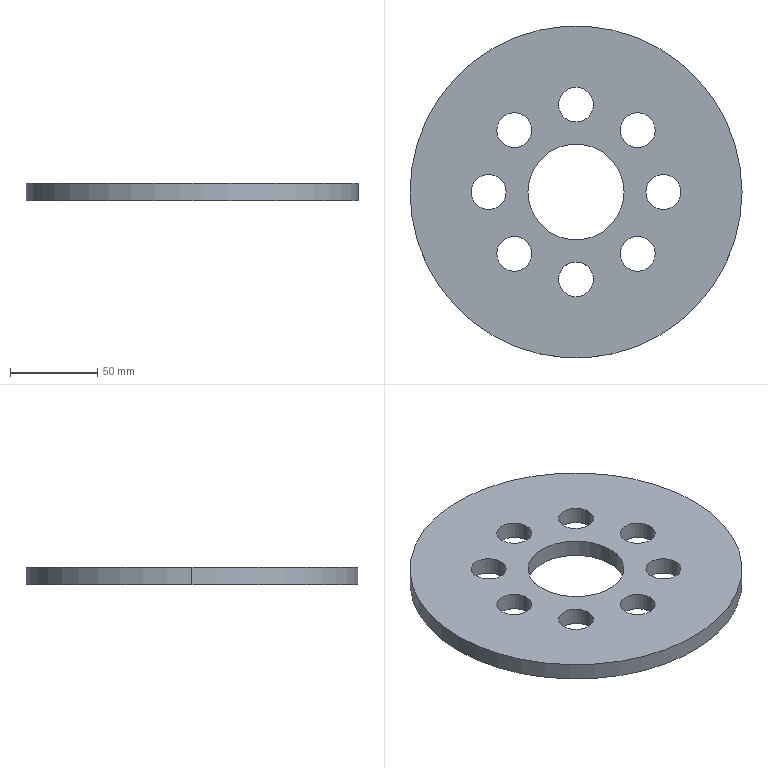Part | SolidWorks | features CirPattern 1, Cut 1, Extrusion 1 | 1 solid | 22 faces | box 190 x 190 x 10 mm | volume 234638 mm3 | cylinder 20 | plane 2 | commonest cylinder face diameters 20 x16 55 x2 190 x2
STEP:
#1=CARTESIAN_POINT('',(-10.,50.,0.));
#2=VERTEX_POINT('',#1);
#3=CARTESIAN_POINT('',(10.,50.,0.));
#4=VERTEX_POINT('',#3);
#5=CARTESIAN_POINT('',(0.,50.,0.));
#6=DIRECTION('',(0.,0.,1.));
#7=DIRECTION('',(0.,1.,0.));
#8=AXIS2_PLACEMENT_3D('',#5,#6,#7);
#9=CIRCLE('',#8,10.);
#10=EDGE_CURVE('',#2,#4,#9,.T.);
#11=ORIENTED_EDGE('',*,*,#10,.F.);
#12=CARTESIAN_POINT('',(-10.,50.,10.));
#13=VERTEX_POINT('',#12);
#14=CARTESIAN_POINT('',(-10.,50.,0.));
#15=DIRECTION('',(0.,0.,1.));
#16=VECTOR('',#15,1000.);
#17=LINE('',#14,#16);
#18=EDGE_CURVE('',#2,#13,#17,.T.);
#19=ORIENTED_EDGE('',*,*,#18,.T.);
#20=CARTESIAN_POINT('',(10.,50.,10.));
#21=VERTEX_POINT('',#20);
#22=CARTESIAN_POINT('',(0.,50.,10.));
#23=DIRECTION('',(0.,0.,1.));
#24=DIRECTION('',(1.,0.,0.));
#25=AXIS2_PLACEMENT_3D('',#22,#23,#24);
#26=CIRCLE('',#25,10.);
#27=EDGE_CURVE('',#13,#21,#26,.T.);
#28=ORIENTED_EDGE('',*,*,#27,.T.);
#29=CARTESIAN_POINT('',(10.,50.,0.));
#30=DIRECTION('',(0.,0.,1.));
#31=VECTOR('',#30,1000.);
#32=LINE('',#29,#31);
#33=EDGE_CURVE('',#4,#21,#32,.T.);
#34=ORIENTED_EDGE('',*,*,#33,.F.);
#35=EDGE_LOOP('',(#11,#19,#28,#34));
#36=FACE_OUTER_BOUND('',#35,.T.);
#37=CARTESIAN_POINT('',(0.,50.,0.));
#38=DIRECTION('',(0.,0.,1.));
#39=DIRECTION('',(1.,0.,0.));
#40=AXIS2_PLACEMENT_3D('',#37,#38,#39);
#41=CYLINDRICAL_SURFACE('',#40,10.);
#42=ADVANCED_FACE('',(#36),#41,.F.);
#43=CARTESIAN_POINT('',(-45.355,35.355,0.));
#44=VERTEX_POINT('',#43);
#45=CARTESIAN_POINT('',(-25.355,35.355,0.));
#46=VERTEX_POINT('',#45);
#47=CARTESIAN_POINT('',(-35.355,35.355,0.));
#48=DIRECTION('',(0.,0.,1.));
#49=DIRECTION('',(-0.7071,0.7071,0.));
#50=AXIS2_PLACEMENT_3D('',#47,#48,#49);
#51=CIRCLE('',#50,10.);
#52=EDGE_CURVE('',#44,#46,#51,.T.);
#53=ORIENTED_EDGE('',*,*,#52,.F.);
#54=CARTESIAN_POINT('',(-45.355,35.355,10.));
#55=VERTEX_POINT('',#54);
#56=CARTESIAN_POINT('',(-45.355,35.355,0.));
#57=DIRECTION('',(0.,0.,1.));
#58=VECTOR('',#57,1000.);
#59=LINE('',#56,#58);
#60=EDGE_CURVE('',#44,#55,#59,.T.);
#61=ORIENTED_EDGE('',*,*,#60,.T.);
#62=CARTESIAN_POINT('',(-25.355,35.355,10.));
#63=VERTEX_POINT('',#62);
#64=CARTESIAN_POINT('',(-35.355,35.355,10.));
#65=DIRECTION('',(0.,0.,1.));
#66=DIRECTION('',(1.,0.,0.));
#67=AXIS2_PLACEMENT_3D('',#64,#65,#66);
#68=CIRCLE('',#67,10.);
#69=EDGE_CURVE('',#55,#63,#68,.T.);
#70=ORIENTED_EDGE('',*,*,#69,.T.);
#71=CARTESIAN_POINT('',(-25.355,35.355,0.));
#72=DIRECTION('',(0.,0.,1.));
#73=VECTOR('',#72,1000.);
#74=LINE('',#71,#73);
#75=EDGE_CURVE('',#46,#63,#74,.T.);
#76=ORIENTED_EDGE('',*,*,#75,.F.);
#77=EDGE_LOOP('',(#53,#61,#70,#76));
#78=FACE_OUTER_BOUND('',#77,.T.);
#79=CARTESIAN_POINT('',(-35.355,35.355,0.));
#80=DIRECTION('',(0.,0.,1.));
#81=DIRECTION('',(1.,0.,0.));
#82=AXIS2_PLACEMENT_3D('',#79,#80,#81);
#83=CYLINDRICAL_SURFACE('',#82,10.);
#84=ADVANCED_FACE('',(#78),#83,.F.);
#85=CARTESIAN_POINT('',(-60.,0.,0.));
#86=VERTEX_POINT('',#85);
#87=CARTESIAN_POINT('',(-40.,0.,0.));
#88=VERTEX_POINT('',#87);
#89=CARTESIAN_POINT('',(-50.,0.,0.));
#90=DIRECTION('',(0.,0.,1.));
#91=DIRECTION('',(-1.,0.,0.));
#92=AXIS2_PLACEMENT_3D('',#89,#90,#91);
#93=CIRCLE('',#92,10.);
#94=EDGE_CURVE('',#86,#88,#93,.T.);
#95=ORIENTED_EDGE('',*,*,#94,.F.);
#96=CARTESIAN_POINT('',(-60.,0.,10.));
#97=VERTEX_POINT('',#96);
#98=CARTESIAN_POINT('',(-60.,0.,0.));
#99=DIRECTION('',(0.,0.,1.));
#100=VECTOR('',#99,1000.);
#101=LINE('',#98,#100);
#102=EDGE_CURVE('',#86,#97,#101,.T.);
#103=ORIENTED_EDGE('',*,*,#102,.T.);
#104=CARTESIAN_POINT('',(-40.,0.,10.));
#105=VERTEX_POINT('',#104);
#106=CARTESIAN_POINT('',(-50.,0.,10.));
#107=DIRECTION('',(0.,0.,1.));
#108=DIRECTION('',(1.,0.,0.));
#109=AXIS2_PLACEMENT_3D('',#106,#107,#108);
#110=CIRCLE('',#109,10.);
#111=EDGE_CURVE('',#97,#105,#110,.T.);
#112=ORIENTED_EDGE('',*,*,#111,.T.);
#113=CARTESIAN_POINT('',(-40.,0.,0.));
#114=DIRECTION('',(0.,0.,1.));
#115=VECTOR('',#114,1000.);
#116=LINE('',#113,#115);
#117=EDGE_CURVE('',#88,#105,#116,.T.);
#118=ORIENTED_EDGE('',*,*,#117,.F.);
#119=EDGE_LOOP('',(#95,#103,#112,#118));
#120=FACE_OUTER_BOUND('',#119,.T.);
#121=CARTESIAN_POINT('',(-50.,0.,0.));
#122=DIRECTION('',(0.,0.,1.));
#123=DIRECTION('',(1.,0.,0.));
#124=AXIS2_PLACEMENT_3D('',#121,#122,#123);
#125=CYLINDRICAL_SURFACE('',#124,10.);
#126=ADVANCED_FACE('',(#120),#125,.F.);
#127=CARTESIAN_POINT('',(-45.355,-35.355,0.));
#128=VERTEX_POINT('',#127);
#129=CARTESIAN_POINT('',(-25.355,-35.355,0.));
#130=VERTEX_POINT('',#129);
#131=CARTESIAN_POINT('',(-35.355,-35.355,0.));
#132=DIRECTION('',(0.,0.,1.));
#133=DIRECTION('',(-0.7071,-0.7071,0.));
#134=AXIS2_PLACEMENT_3D('',#131,#132,#133);
#135=CIRCLE('',#134,10.);
#136=EDGE_CURVE('',#128,#130,#135,.T.);
#137=ORIENTED_EDGE('',*,*,#136,.F.);
#138=CARTESIAN_POINT('',(-45.355,-35.355,10.));
#139=VERTEX_POINT('',#138);
#140=CARTESIAN_POINT('',(-45.355,-35.355,0.));
#141=DIRECTION('',(0.,0.,1.));
#142=VECTOR('',#141,1000.);
#143=LINE('',#140,#142);
#144=EDGE_CURVE('',#128,#139,#143,.T.);
#145=ORIENTED_EDGE('',*,*,#144,.T.);
#146=CARTESIAN_POINT('',(-25.355,-35.355,10.));
#147=VERTEX_POINT('',#146);
#148=CARTESIAN_POINT('',(-35.355,-35.355,10.));
#149=DIRECTION('',(0.,0.,1.));
#150=DIRECTION('',(1.,0.,0.));
#151=AXIS2_PLACEMENT_3D('',#148,#149,#150);
#152=CIRCLE('',#151,10.);
#153=EDGE_CURVE('',#139,#147,#152,.T.);
#154=ORIENTED_EDGE('',*,*,#153,.T.);
#155=CARTESIAN_POINT('',(-25.355,-35.355,0.));
#156=DIRECTION('',(0.,0.,1.));
#157=VECTOR('',#156,1000.);
#158=LINE('',#155,#157);
#159=EDGE_CURVE('',#130,#147,#158,.T.);
#160=ORIENTED_EDGE('',*,*,#159,.F.);
#161=EDGE_LOOP('',(#137,#145,#154,#160));
#162=FACE_OUTER_BOUND('',#161,.T.);
#163=CARTESIAN_POINT('',(-35.355,-35.355,0.));
#164=DIRECTION('',(0.,0.,1.));
#165=DIRECTION('',(1.,0.,0.));
#166=AXIS2_PLACEMENT_3D('',#163,#164,#165);
#167=CYLINDRICAL_SURFACE('',#166,10.);
#168=ADVANCED_FACE('',(#162),#167,.F.);
#169=CARTESIAN_POINT('',(-10.,-50.,0.));
#170=VERTEX_POINT('',#169);
#171=CARTESIAN_POINT('',(10.,-50.,0.));
#172=VERTEX_POINT('',#171);
#173=CARTESIAN_POINT('',(0.,-50.,0.));
#174=DIRECTION('',(0.,0.,1.));
#175=DIRECTION('',(0.,-1.,0.));
#176=AXIS2_PLACEMENT_3D('',#173,#174,#175);
#177=CIRCLE('',#176,10.);
#178=EDGE_CURVE('',#170,#172,#177,.T.);
#179=ORIENTED_EDGE('',*,*,#178,.F.);
#180=CARTESIAN_POINT('',(-10.,-50.,10.));
#181=VERTEX_POINT('',#180);
#182=CARTESIAN_POINT('',(-10.,-50.,0.));
#183=DIRECTION('',(0.,0.,1.));
#184=VECTOR('',#183,1000.);
#185=LINE('',#182,#184);
#186=EDGE_CURVE('',#170,#181,#185,.T.);
#187=ORIENTED_EDGE('',*,*,#186,.T.);
#188=CARTESIAN_POINT('',(10.,-50.,10.));
#189=VERTEX_POINT('',#188);
#190=CARTESIAN_POINT('',(0.,-50.,10.));
#191=DIRECTION('',(0.,0.,1.));
#192=DIRECTION('',(1.,0.,0.));
#193=AXIS2_PLACEMENT_3D('',#190,#191,#192);
#194=CIRCLE('',#193,10.);
#195=EDGE_CURVE('',#181,#189,#194,.T.);
#196=ORIENTED_EDGE('',*,*,#195,.T.);
#197=CARTESIAN_POINT('',(10.,-50.,0.));
#198=DIRECTION('',(0.,0.,1.));
#199=VECTOR('',#198,1000.);
#200=LINE('',#197,#199);
#201=EDGE_CURVE('',#172,#189,#200,.T.);
#202=ORIENTED_EDGE('',*,*,#201,.F.);
#203=EDGE_LOOP('',(#179,#187,#196,#202));
#204=FACE_OUTER_BOUND('',#203,.T.);
#205=CARTESIAN_POINT('',(0.,-50.,0.));
#206=DIRECTION('',(0.,0.,1.));
#207=DIRECTION('',(1.,0.,0.));
#208=AXIS2_PLACEMENT_3D('',#205,#206,#207);
#209=CYLINDRICAL_SURFACE('',#208,10.);
#210=ADVANCED_FACE('',(#204),#209,.F.);
#211=CARTESIAN_POINT('',(25.355,-35.355,0.));
#212=VERTEX_POINT('',#211);
#213=CARTESIAN_POINT('',(45.355,-35.355,0.));
#214=VERTEX_POINT('',#213);
#215=CARTESIAN_POINT('',(35.355,-35.355,0.));
#216=DIRECTION('',(0.,0.,1.));
#217=DIRECTION('',(0.7071,-0.7071,0.));
#218=AXIS2_PLACEMENT_3D('',#215,#216,#217);
#219=CIRCLE('',#218,10.);
#220=EDGE_CURVE('',#212,#214,#219,.T.);
#221=ORIENTED_EDGE('',*,*,#220,.F.);
#222=CARTESIAN_POINT('',(25.355,-35.355,10.));
#223=VERTEX_POINT('',#222);
#224=CARTESIAN_POINT('',(25.355,-35.355,0.));
#225=DIRECTION('',(0.,0.,1.));
#226=VECTOR('',#225,1000.);
#227=LINE('',#224,#226);
#228=EDGE_CURVE('',#212,#223,#227,.T.);
#229=ORIENTED_EDGE('',*,*,#228,.T.);
#230=CARTESIAN_POINT('',(45.355,-35.355,10.));
#231=VERTEX_POINT('',#230);
#232=CARTESIAN_POINT('',(35.355,-35.355,10.));
#233=DIRECTION('',(0.,0.,1.));
#234=DIRECTION('',(1.,0.,0.));
#235=AXIS2_PLACEMENT_3D('',#232,#233,#234);
#236=CIRCLE('',#235,10.);
#237=EDGE_CURVE('',#223,#231,#236,.T.);
#238=ORIENTED_EDGE('',*,*,#237,.T.);
#239=CARTESIAN_POINT('',(45.355,-35.355,0.));
#240=DIRECTION('',(0.,0.,1.));
#241=VECTOR('',#240,1000.);
#242=LINE('',#239,#241);
#243=EDGE_CURVE('',#214,#231,#242,.T.);
#244=ORIENTED_EDGE('',*,*,#243,.F.);
#245=EDGE_LOOP('',(#221,#229,#238,#244));
#246=FACE_OUTER_BOUND('',#245,.T.);
#247=CARTESIAN_POINT('',(35.355,-35.355,0.));
#248=DIRECTION('',(0.,0.,1.));
#249=DIRECTION('',(1.,0.,0.));
#250=AXIS2_PLACEMENT_3D('',#247,#248,#249);
#251=CYLINDRICAL_SURFACE('',#250,10.);
#252=ADVANCED_FACE('',(#246),#251,.F.);
#253=CARTESIAN_POINT('',(25.355,35.355,0.));
#254=VERTEX_POINT('',#253);
#255=CARTESIAN_POINT('',(45.355,35.355,0.));
#256=VERTEX_POINT('',#255);
#257=CARTESIAN_POINT('',(35.355,35.355,0.));
#258=DIRECTION('',(0.,0.,1.));
#259=DIRECTION('',(0.7071,0.7071,0.));
#260=AXIS2_PLACEMENT_3D('',#257,#258,#259);
#261=CIRCLE('',#260,10.);
#262=EDGE_CURVE('',#254,#256,#261,.T.);
#263=ORIENTED_EDGE('',*,*,#262,.F.);
#264=CARTESIAN_POINT('',(25.355,35.355,10.));
#265=VERTEX_POINT('',#264);
#266=CARTESIAN_POINT('',(25.355,35.355,0.));
#267=DIRECTION('',(0.,0.,1.));
#268=VECTOR('',#267,1000.);
#269=LINE('',#266,#268);
#270=EDGE_CURVE('',#254,#265,#269,.T.);
#271=ORIENTED_EDGE('',*,*,#270,.T.);
#272=CARTESIAN_POINT('',(45.355,35.355,10.));
#273=VERTEX_POINT('',#272);
#274=CARTESIAN_POINT('',(35.355,35.355,10.));
#275=DIRECTION('',(0.,0.,1.));
#276=DIRECTION('',(1.,0.,0.));
#277=AXIS2_PLACEMENT_3D('',#274,#275,#276);
#278=CIRCLE('',#277,10.);
#279=EDGE_CURVE('',#265,#273,#278,.T.);
#280=ORIENTED_EDGE('',*,*,#279,.T.);
#281=CARTESIAN_POINT('',(45.355,35.355,0.));
#282=DIRECTION('',(0.,0.,1.));
#283=VECTOR('',#282,1000.);
#284=LINE('',#281,#283);
#285=EDGE_CURVE('',#256,#273,#284,.T.);
#286=ORIENTED_EDGE('',*,*,#285,.F.);
#287=EDGE_LOOP('',(#263,#271,#280,#286));
#288=FACE_OUTER_BOUND('',#287,.T.);
#289=CARTESIAN_POINT('',(35.355,35.355,0.));
#290=DIRECTION('',(0.,0.,1.));
#291=DIRECTION('',(1.,0.,0.));
#292=AXIS2_PLACEMENT_3D('',#289,#290,#291);
#293=CYLINDRICAL_SURFACE('',#292,10.);
#294=ADVANCED_FACE('',(#288),#293,.F.);
#295=CARTESIAN_POINT('',(40.,0.,0.));
#296=VERTEX_POINT('',#295);
#297=CARTESIAN_POINT('',(60.,0.,0.));
#298=VERTEX_POINT('',#297);
#299=CARTESIAN_POINT('',(50.,0.,0.));
#300=DIRECTION('',(0.,0.,1.));
#301=DIRECTION('',(1.,0.,0.));
#302=AXIS2_PLACEMENT_3D('',#299,#300,#301);
#303=CIRCLE('',#302,10.);
#304=EDGE_CURVE('',#296,#298,#303,.T.);
#305=ORIENTED_EDGE('',*,*,#304,.F.);
#306=CARTESIAN_POINT('',(40.,0.,10.));
#307=VERTEX_POINT('',#306);
#308=CARTESIAN_POINT('',(40.,0.,0.));
#309=DIRECTION('',(0.,0.,1.));
#310=VECTOR('',#309,1000.);
#311=LINE('',#308,#310);
#312=EDGE_CURVE('',#296,#307,#311,.T.);
#313=ORIENTED_EDGE('',*,*,#312,.T.);
#314=CARTESIAN_POINT('',(60.,0.,10.));
#315=VERTEX_POINT('',#314);
#316=CARTESIAN_POINT('',(50.,0.,10.));
#317=DIRECTION('',(0.,0.,1.));
#318=DIRECTION('',(1.,0.,0.));
#319=AXIS2_PLACEMENT_3D('',#316,#317,#318);
#320=CIRCLE('',#319,10.);
#321=EDGE_CURVE('',#307,#315,#320,.T.);
#322=ORIENTED_EDGE('',*,*,#321,.T.);
#323=CARTESIAN_POINT('',(60.,0.,0.));
#324=DIRECTION('',(0.,0.,1.));
#325=VECTOR('',#324,1000.);
#326=LINE('',#323,#325);
#327=EDGE_CURVE('',#298,#315,#326,.T.);
#328=ORIENTED_EDGE('',*,*,#327,.F.);
#329=EDGE_LOOP('',(#305,#313,#322,#328));
#330=FACE_OUTER_BOUND('',#329,.T.);
#331=CARTESIAN_POINT('',(50.,0.,0.));
#332=DIRECTION('',(0.,0.,1.));
#333=DIRECTION('',(1.,0.,0.));
#334=AXIS2_PLACEMENT_3D('',#331,#332,#333);
#335=CYLINDRICAL_SURFACE('',#334,10.);
#336=ADVANCED_FACE('',(#330),#335,.F.);
#337=CARTESIAN_POINT('',(-27.5,0.,10.));
#338=VERTEX_POINT('',#337);
#339=CARTESIAN_POINT('',(27.5,0.,10.));
#340=VERTEX_POINT('',#339);
#341=CARTESIAN_POINT('',(0.,0.,10.));
#342=DIRECTION('',(0.,0.,1.));
#343=DIRECTION('',(1.,0.,0.));
#344=AXIS2_PLACEMENT_3D('',#341,#342,#343);
#345=CIRCLE('',#344,27.5);
#346=EDGE_CURVE('',#338,#340,#345,.T.);
#347=ORIENTED_EDGE('',*,*,#346,.T.);
#348=CARTESIAN_POINT('',(27.5,0.,0.));
#349=VERTEX_POINT('',#348);
#350=CARTESIAN_POINT('',(27.5,0.,10.));
#351=DIRECTION('',(0.,0.,-1.));
#352=VECTOR('',#351,1000.);
#353=LINE('',#350,#352);
#354=EDGE_CURVE('',#340,#349,#353,.T.);
#355=ORIENTED_EDGE('',*,*,#354,.T.);
#356=CARTESIAN_POINT('',(-27.5,0.,0.));
#357=VERTEX_POINT('',#356);
#358=CARTESIAN_POINT('',(0.,0.,0.));
#359=DIRECTION('',(0.,0.,1.));
#360=DIRECTION('',(1.,0.,0.));
#361=AXIS2_PLACEMENT_3D('',#358,#359,#360);
#362=CIRCLE('',#361,27.5);
#363=EDGE_CURVE('',#357,#349,#362,.T.);
#364=ORIENTED_EDGE('',*,*,#363,.F.);
#365=CARTESIAN_POINT('',(-27.5,0.,10.));
#366=DIRECTION('',(0.,0.,-1.));
#367=VECTOR('',#366,1000.);
#368=LINE('',#365,#367);
#369=EDGE_CURVE('',#338,#357,#368,.T.);
#370=ORIENTED_EDGE('',*,*,#369,.F.);
#371=EDGE_LOOP('',(#347,#355,#364,#370));
#372=FACE_OUTER_BOUND('',#371,.T.);
#373=CARTESIAN_POINT('',(0.,0.,10.));
#374=DIRECTION('',(0.,0.,-1.));
#375=DIRECTION('',(-1.,0.,0.));
#376=AXIS2_PLACEMENT_3D('',#373,#374,#375);
#377=CYLINDRICAL_SURFACE('',#376,27.5);
#378=ADVANCED_FACE('',(#372),#377,.F.);
#379=CARTESIAN_POINT('',(95.,0.,10.));
#380=VERTEX_POINT('',#379);
#381=CARTESIAN_POINT('',(-95.,0.,10.));
#382=VERTEX_POINT('',#381);
#383=CARTESIAN_POINT('',(0.,0.,10.));
#384=DIRECTION('',(0.,0.,1.));
#385=DIRECTION('',(1.,0.,0.));
#386=AXIS2_PLACEMENT_3D('',#383,#384,#385);
#387=CIRCLE('',#386,95.);
#388=EDGE_CURVE('',#380,#382,#387,.T.);
#389=ORIENTED_EDGE('',*,*,#388,.F.);
#390=CARTESIAN_POINT('',(95.,0.,0.));
#391=VERTEX_POINT('',#390);
#392=CARTESIAN_POINT('',(95.,0.,10.));
#393=DIRECTION('',(0.,0.,-1.));
#394=VECTOR('',#393,1000.);
#395=LINE('',#392,#394);
#396=EDGE_CURVE('',#380,#391,#395,.T.);
#397=ORIENTED_EDGE('',*,*,#396,.T.);
#398=CARTESIAN_POINT('',(-95.,0.,0.));
#399=VERTEX_POINT('',#398);
#400=CARTESIAN_POINT('',(0.,0.,0.));
#401=DIRECTION('',(0.,0.,1.));
#402=DIRECTION('',(1.,0.,0.));
#403=AXIS2_PLACEMENT_3D('',#400,#401,#402);
#404=CIRCLE('',#403,95.);
#405=EDGE_CURVE('',#391,#399,#404,.T.);
#406=ORIENTED_EDGE('',*,*,#405,.T.);
#407=CARTESIAN_POINT('',(-95.,0.,10.));
#408=DIRECTION('',(0.,0.,-1.));
#409=VECTOR('',#408,1000.);
#410=LINE('',#407,#409);
#411=EDGE_CURVE('',#382,#399,#410,.T.);
#412=ORIENTED_EDGE('',*,*,#411,.F.);
#413=EDGE_LOOP('',(#389,#397,#406,#412));
#414=FACE_OUTER_BOUND('',#413,.T.);
#415=CARTESIAN_POINT('',(0.,0.,10.));
#416=DIRECTION('',(0.,0.,-1.));
#417=DIRECTION('',(-1.,0.,0.));
#418=AXIS2_PLACEMENT_3D('',#415,#416,#417);
#419=CYLINDRICAL_SURFACE('',#418,95.);
#420=ADVANCED_FACE('',(#414),#419,.T.);
#421=CARTESIAN_POINT('',(0.,50.,10.));
#422=DIRECTION('',(0.,0.,1.));
#423=DIRECTION('',(1.,0.,0.));
#424=AXIS2_PLACEMENT_3D('',#421,#422,#423);
#425=CIRCLE('',#424,10.);
#426=EDGE_CURVE('',#21,#13,#425,.T.);
#427=ORIENTED_EDGE('',*,*,#426,.F.);
#428=ORIENTED_EDGE('',*,*,#27,.F.);
#429=EDGE_LOOP('',(#427,#428));
#430=FACE_BOUND('',#429,.T.);
#431=CARTESIAN_POINT('',(-35.355,35.355,10.));
#432=DIRECTION('',(0.,0.,1.));
#433=DIRECTION('',(1.,0.,0.));
#434=AXIS2_PLACEMENT_3D('',#431,#432,#433);
#435=CIRCLE('',#434,10.);
#436=EDGE_CURVE('',#63,#55,#435,.T.);
#437=ORIENTED_EDGE('',*,*,#436,.F.);
#438=ORIENTED_EDGE('',*,*,#69,.F.);
#439=EDGE_LOOP('',(#437,#438));
#440=FACE_BOUND('',#439,.T.);
#441=CARTESIAN_POINT('',(-50.,0.,10.));
#442=DIRECTION('',(0.,0.,1.));
#443=DIRECTION('',(1.,0.,0.));
#444=AXIS2_PLACEMENT_3D('',#441,#442,#443);
#445=CIRCLE('',#444,10.);
#446=EDGE_CURVE('',#105,#97,#445,.T.);
#447=ORIENTED_EDGE('',*,*,#446,.F.);
#448=ORIENTED_EDGE('',*,*,#111,.F.);
#449=EDGE_LOOP('',(#447,#448));
#450=FACE_BOUND('',#449,.T.);
#451=CARTESIAN_POINT('',(-35.355,-35.355,10.));
#452=DIRECTION('',(0.,0.,1.));
#453=DIRECTION('',(1.,0.,0.));
#454=AXIS2_PLACEMENT_3D('',#451,#452,#453);
#455=CIRCLE('',#454,10.);
#456=EDGE_CURVE('',#147,#139,#455,.T.);
#457=ORIENTED_EDGE('',*,*,#456,.F.);
#458=ORIENTED_EDGE('',*,*,#153,.F.);
#459=EDGE_LOOP('',(#457,#458));
#460=FACE_BOUND('',#459,.T.);
#461=CARTESIAN_POINT('',(0.,-50.,10.));
#462=DIRECTION('',(0.,0.,1.));
#463=DIRECTION('',(1.,0.,0.));
#464=AXIS2_PLACEMENT_3D('',#461,#462,#463);
#465=CIRCLE('',#464,10.);
#466=EDGE_CURVE('',#189,#181,#465,.T.);
#467=ORIENTED_EDGE('',*,*,#466,.F.);
#468=ORIENTED_EDGE('',*,*,#195,.F.);
#469=EDGE_LOOP('',(#467,#468));
#470=FACE_BOUND('',#469,.T.);
#471=CARTESIAN_POINT('',(35.355,-35.355,10.));
#472=DIRECTION('',(0.,0.,1.));
#473=DIRECTION('',(1.,0.,0.));
#474=AXIS2_PLACEMENT_3D('',#471,#472,#473);
#475=CIRCLE('',#474,10.);
#476=EDGE_CURVE('',#231,#223,#475,.T.);
#477=ORIENTED_EDGE('',*,*,#476,.F.);
#478=ORIENTED_EDGE('',*,*,#237,.F.);
#479=EDGE_LOOP('',(#477,#478));
#480=FACE_BOUND('',#479,.T.);
#481=CARTESIAN_POINT('',(35.355,35.355,10.));
#482=DIRECTION('',(0.,0.,1.));
#483=DIRECTION('',(1.,0.,0.));
#484=AXIS2_PLACEMENT_3D('',#481,#482,#483);
#485=CIRCLE('',#484,10.);
#486=EDGE_CURVE('',#273,#265,#485,.T.);
#487=ORIENTED_EDGE('',*,*,#486,.F.);
#488=ORIENTED_EDGE('',*,*,#279,.F.);
#489=EDGE_LOOP('',(#487,#488));
#490=FACE_BOUND('',#489,.T.);
#491=CARTESIAN_POINT('',(50.,0.,10.));
#492=DIRECTION('',(0.,0.,1.));
#493=DIRECTION('',(1.,0.,0.));
#494=AXIS2_PLACEMENT_3D('',#491,#492,#493);
#495=CIRCLE('',#494,10.);
#496=EDGE_CURVE('',#315,#307,#495,.T.);
#497=ORIENTED_EDGE('',*,*,#496,.F.);
#498=ORIENTED_EDGE('',*,*,#321,.F.);
#499=EDGE_LOOP('',(#497,#498));
#500=FACE_BOUND('',#499,.T.);
#501=CARTESIAN_POINT('',(0.,0.,10.));
#502=DIRECTION('',(0.,0.,1.));
#503=DIRECTION('',(1.,0.,0.));
#504=AXIS2_PLACEMENT_3D('',#501,#502,#503);
#505=CIRCLE('',#504,95.);
#506=EDGE_CURVE('',#382,#380,#505,.T.);
#507=ORIENTED_EDGE('',*,*,#506,.T.);
#508=ORIENTED_EDGE('',*,*,#388,.T.);
#509=EDGE_LOOP('',(#507,#508));
#510=FACE_OUTER_BOUND('',#509,.T.);
#511=ORIENTED_EDGE('',*,*,#346,.F.);
#512=CARTESIAN_POINT('',(0.,0.,10.));
#513=DIRECTION('',(0.,0.,1.));
#514=DIRECTION('',(1.,0.,0.));
#515=AXIS2_PLACEMENT_3D('',#512,#513,#514);
#516=CIRCLE('',#515,27.5);
#517=EDGE_CURVE('',#340,#338,#516,.T.);
#518=ORIENTED_EDGE('',*,*,#517,.F.);
#519=EDGE_LOOP('',(#511,#518));
#520=FACE_BOUND('',#519,.T.);
#521=CARTESIAN_POINT('',(0.,0.,10.));
#522=DIRECTION('',(0.,0.,1.));
#523=DIRECTION('',(1.,0.,0.));
#524=AXIS2_PLACEMENT_3D('',#521,#522,#523);
#525=PLANE('',#524);
#526=ADVANCED_FACE('',(#430,#440,#450,#460,#470,#480,#490,#500,#510,#520),#525,.T.);
#527=CARTESIAN_POINT('',(0.,50.,0.));
#528=DIRECTION('',(0.,0.,1.));
#529=DIRECTION('',(0.,1.,0.));
#530=AXIS2_PLACEMENT_3D('',#527,#528,#529);
#531=CIRCLE('',#530,10.);
#532=EDGE_CURVE('',#4,#2,#531,.T.);
#533=ORIENTED_EDGE('',*,*,#532,.T.);
#534=ORIENTED_EDGE('',*,*,#10,.T.);
#535=EDGE_LOOP('',(#533,#534));
#536=FACE_BOUND('',#535,.T.);
#537=CARTESIAN_POINT('',(-35.355,35.355,0.));
#538=DIRECTION('',(0.,0.,1.));
#539=DIRECTION('',(-0.7071,0.7071,0.));
#540=AXIS2_PLACEMENT_3D('',#537,#538,#539);
#541=CIRCLE('',#540,10.);
#542=EDGE_CURVE('',#46,#44,#541,.T.);
#543=ORIENTED_EDGE('',*,*,#542,.T.);
#544=ORIENTED_EDGE('',*,*,#52,.T.);
#545=EDGE_LOOP('',(#543,#544));
#546=FACE_BOUND('',#545,.T.);
#547=CARTESIAN_POINT('',(-50.,0.,0.));
#548=DIRECTION('',(0.,0.,1.));
#549=DIRECTION('',(-1.,0.,0.));
#550=AXIS2_PLACEMENT_3D('',#547,#548,#549);
#551=CIRCLE('',#550,10.);
#552=EDGE_CURVE('',#88,#86,#551,.T.);
#553=ORIENTED_EDGE('',*,*,#552,.T.);
#554=ORIENTED_EDGE('',*,*,#94,.T.);
#555=EDGE_LOOP('',(#553,#554));
#556=FACE_BOUND('',#555,.T.);
#557=CARTESIAN_POINT('',(-35.355,-35.355,0.));
#558=DIRECTION('',(0.,0.,1.));
#559=DIRECTION('',(-0.7071,-0.7071,0.));
#560=AXIS2_PLACEMENT_3D('',#557,#558,#559);
#561=CIRCLE('',#560,10.);
#562=EDGE_CURVE('',#130,#128,#561,.T.);
#563=ORIENTED_EDGE('',*,*,#562,.T.);
#564=ORIENTED_EDGE('',*,*,#136,.T.);
#565=EDGE_LOOP('',(#563,#564));
#566=FACE_BOUND('',#565,.T.);
#567=CARTESIAN_POINT('',(0.,-50.,0.));
#568=DIRECTION('',(0.,0.,1.));
#569=DIRECTION('',(0.,-1.,0.));
#570=AXIS2_PLACEMENT_3D('',#567,#568,#569);
#571=CIRCLE('',#570,10.);
#572=EDGE_CURVE('',#172,#170,#571,.T.);
#573=ORIENTED_EDGE('',*,*,#572,.T.);
#574=ORIENTED_EDGE('',*,*,#178,.T.);
#575=EDGE_LOOP('',(#573,#574));
#576=FACE_BOUND('',#575,.T.);
#577=CARTESIAN_POINT('',(35.355,-35.355,0.));
#578=DIRECTION('',(0.,0.,1.));
#579=DIRECTION('',(0.7071,-0.7071,0.));
#580=AXIS2_PLACEMENT_3D('',#577,#578,#579);
#581=CIRCLE('',#580,10.);
#582=EDGE_CURVE('',#214,#212,#581,.T.);
#583=ORIENTED_EDGE('',*,*,#582,.T.);
#584=ORIENTED_EDGE('',*,*,#220,.T.);
#585=EDGE_LOOP('',(#583,#584));
#586=FACE_BOUND('',#585,.T.);
#587=CARTESIAN_POINT('',(35.355,35.355,0.));
#588=DIRECTION('',(0.,0.,1.));
#589=DIRECTION('',(0.7071,0.7071,0.));
#590=AXIS2_PLACEMENT_3D('',#587,#588,#589);
#591=CIRCLE('',#590,10.);
#592=EDGE_CURVE('',#256,#254,#591,.T.);
#593=ORIENTED_EDGE('',*,*,#592,.T.);
#594=ORIENTED_EDGE('',*,*,#262,.T.);
#595=EDGE_LOOP('',(#593,#594));
#596=FACE_BOUND('',#595,.T.);
#597=CARTESIAN_POINT('',(50.,0.,0.));
#598=DIRECTION('',(0.,0.,1.));
#599=DIRECTION('',(1.,0.,0.));
#600=AXIS2_PLACEMENT_3D('',#597,#598,#599);
#601=CIRCLE('',#600,10.);
#602=EDGE_CURVE('',#298,#296,#601,.T.);
#603=ORIENTED_EDGE('',*,*,#602,.T.);
#604=ORIENTED_EDGE('',*,*,#304,.T.);
#605=EDGE_LOOP('',(#603,#604));
#606=FACE_BOUND('',#605,.T.);
#607=CARTESIAN_POINT('',(0.,0.,0.));
#608=DIRECTION('',(0.,0.,1.));
#609=DIRECTION('',(1.,0.,0.));
#610=AXIS2_PLACEMENT_3D('',#607,#608,#609);
#611=CIRCLE('',#610,95.);
#612=EDGE_CURVE('',#399,#391,#611,.T.);
#613=ORIENTED_EDGE('',*,*,#612,.F.);
#614=ORIENTED_EDGE('',*,*,#405,.F.);
#615=EDGE_LOOP('',(#613,#614));
#616=FACE_OUTER_BOUND('',#615,.T.);
#617=ORIENTED_EDGE('',*,*,#363,.T.);
#618=CARTESIAN_POINT('',(0.,0.,0.));
#619=DIRECTION('',(0.,0.,1.));
#620=DIRECTION('',(1.,0.,0.));
#621=AXIS2_PLACEMENT_3D('',#618,#619,#620);
#622=CIRCLE('',#621,27.5);
#623=EDGE_CURVE('',#349,#357,#622,.T.);
#624=ORIENTED_EDGE('',*,*,#623,.T.);
#625=EDGE_LOOP('',(#617,#624));
#626=FACE_BOUND('',#625,.T.);
#627=CARTESIAN_POINT('',(0.,0.,0.));
#628=DIRECTION('',(0.,0.,1.));
#629=DIRECTION('',(1.,0.,0.));
#630=AXIS2_PLACEMENT_3D('',#627,#628,#629);
#631=PLANE('',#630);
#632=ADVANCED_FACE('',(#536,#546,#556,#566,#576,#586,#596,#606,#616,#626),#631,.F.);
#633=ORIENTED_EDGE('',*,*,#396,.F.);
#634=ORIENTED_EDGE('',*,*,#506,.F.);
#635=ORIENTED_EDGE('',*,*,#411,.T.);
#636=ORIENTED_EDGE('',*,*,#612,.T.);
#637=EDGE_LOOP('',(#633,#634,#635,#636));
#638=FACE_OUTER_BOUND('',#637,.T.);
#639=CARTESIAN_POINT('',(0.,0.,10.));
#640=DIRECTION('',(0.,0.,-1.));
#641=DIRECTION('',(-1.,0.,0.));
#642=AXIS2_PLACEMENT_3D('',#639,#640,#641);
#643=CYLINDRICAL_SURFACE('',#642,95.);
#644=ADVANCED_FACE('',(#638),#643,.T.);
#645=ORIENTED_EDGE('',*,*,#354,.F.);
#646=ORIENTED_EDGE('',*,*,#517,.T.);
#647=ORIENTED_EDGE('',*,*,#369,.T.);
#648=ORIENTED_EDGE('',*,*,#623,.F.);
#649=EDGE_LOOP('',(#645,#646,#647,#648));
#650=FACE_OUTER_BOUND('',#649,.T.);
#651=CARTESIAN_POINT('',(0.,0.,10.));
#652=DIRECTION('',(0.,0.,-1.));
#653=DIRECTION('',(-1.,0.,0.));
#654=AXIS2_PLACEMENT_3D('',#651,#652,#653);
#655=CYLINDRICAL_SURFACE('',#654,27.5);
#656=ADVANCED_FACE('',(#650),#655,.F.);
#657=ORIENTED_EDGE('',*,*,#312,.F.);
#658=ORIENTED_EDGE('',*,*,#602,.F.);
#659=ORIENTED_EDGE('',*,*,#327,.T.);
#660=ORIENTED_EDGE('',*,*,#496,.T.);
#661=EDGE_LOOP('',(#657,#658,#659,#660));
#662=FACE_OUTER_BOUND('',#661,.T.);
#663=CARTESIAN_POINT('',(50.,0.,0.));
#664=DIRECTION('',(0.,0.,1.));
#665=DIRECTION('',(1.,0.,0.));
#666=AXIS2_PLACEMENT_3D('',#663,#664,#665);
#667=CYLINDRICAL_SURFACE('',#666,10.);
#668=ADVANCED_FACE('',(#662),#667,.F.);
#669=ORIENTED_EDGE('',*,*,#270,.F.);
#670=ORIENTED_EDGE('',*,*,#592,.F.);
#671=ORIENTED_EDGE('',*,*,#285,.T.);
#672=ORIENTED_EDGE('',*,*,#486,.T.);
#673=EDGE_LOOP('',(#669,#670,#671,#672));
#674=FACE_OUTER_BOUND('',#673,.T.);
#675=CARTESIAN_POINT('',(35.355,35.355,0.));
#676=DIRECTION('',(0.,0.,1.));
#677=DIRECTION('',(1.,0.,0.));
#678=AXIS2_PLACEMENT_3D('',#675,#676,#677);
#679=CYLINDRICAL_SURFACE('',#678,10.);
#680=ADVANCED_FACE('',(#674),#679,.F.);
#681=ORIENTED_EDGE('',*,*,#228,.F.);
#682=ORIENTED_EDGE('',*,*,#582,.F.);
#683=ORIENTED_EDGE('',*,*,#243,.T.);
#684=ORIENTED_EDGE('',*,*,#476,.T.);
#685=EDGE_LOOP('',(#681,#682,#683,#684));
#686=FACE_OUTER_BOUND('',#685,.T.);
#687=CARTESIAN_POINT('',(35.355,-35.355,0.));
#688=DIRECTION('',(0.,0.,1.));
#689=DIRECTION('',(1.,0.,0.));
#690=AXIS2_PLACEMENT_3D('',#687,#688,#689);
#691=CYLINDRICAL_SURFACE('',#690,10.);
#692=ADVANCED_FACE('',(#686),#691,.F.);
#693=ORIENTED_EDGE('',*,*,#186,.F.);
#694=ORIENTED_EDGE('',*,*,#572,.F.);
#695=ORIENTED_EDGE('',*,*,#201,.T.);
#696=ORIENTED_EDGE('',*,*,#466,.T.);
#697=EDGE_LOOP('',(#693,#694,#695,#696));
#698=FACE_OUTER_BOUND('',#697,.T.);
#699=CARTESIAN_POINT('',(0.,-50.,0.));
#700=DIRECTION('',(0.,0.,1.));
#701=DIRECTION('',(1.,0.,0.));
#702=AXIS2_PLACEMENT_3D('',#699,#700,#701);
#703=CYLINDRICAL_SURFACE('',#702,10.);
#704=ADVANCED_FACE('',(#698),#703,.F.);
#705=ORIENTED_EDGE('',*,*,#144,.F.);
#706=ORIENTED_EDGE('',*,*,#562,.F.);
#707=ORIENTED_EDGE('',*,*,#159,.T.);
#708=ORIENTED_EDGE('',*,*,#456,.T.);
#709=EDGE_LOOP('',(#705,#706,#707,#708));
#710=FACE_OUTER_BOUND('',#709,.T.);
#711=CARTESIAN_POINT('',(-35.355,-35.355,0.));
#712=DIRECTION('',(0.,0.,1.));
#713=DIRECTION('',(1.,0.,0.));
#714=AXIS2_PLACEMENT_3D('',#711,#712,#713);
#715=CYLINDRICAL_SURFACE('',#714,10.);
#716=ADVANCED_FACE('',(#710),#715,.F.);
#717=ORIENTED_EDGE('',*,*,#102,.F.);
#718=ORIENTED_EDGE('',*,*,#552,.F.);
#719=ORIENTED_EDGE('',*,*,#117,.T.);
#720=ORIENTED_EDGE('',*,*,#446,.T.);
#721=EDGE_LOOP('',(#717,#718,#719,#720));
#722=FACE_OUTER_BOUND('',#721,.T.);
#723=CARTESIAN_POINT('',(-50.,0.,0.));
#724=DIRECTION('',(0.,0.,1.));
#725=DIRECTION('',(1.,0.,0.));
#726=AXIS2_PLACEMENT_3D('',#723,#724,#725);
#727=CYLINDRICAL_SURFACE('',#726,10.);
#728=ADVANCED_FACE('',(#722),#727,.F.);
#729=ORIENTED_EDGE('',*,*,#60,.F.);
#730=ORIENTED_EDGE('',*,*,#542,.F.);
#731=ORIENTED_EDGE('',*,*,#75,.T.);
#732=ORIENTED_EDGE('',*,*,#436,.T.);
#733=EDGE_LOOP('',(#729,#730,#731,#732));
#734=FACE_OUTER_BOUND('',#733,.T.);
#735=CARTESIAN_POINT('',(-35.355,35.355,0.));
#736=DIRECTION('',(0.,0.,1.));
#737=DIRECTION('',(1.,0.,0.));
#738=AXIS2_PLACEMENT_3D('',#735,#736,#737);
#739=CYLINDRICAL_SURFACE('',#738,10.);
#740=ADVANCED_FACE('',(#734),#739,.F.);
#741=ORIENTED_EDGE('',*,*,#18,.F.);
#742=ORIENTED_EDGE('',*,*,#532,.F.);
#743=ORIENTED_EDGE('',*,*,#33,.T.);
#744=ORIENTED_EDGE('',*,*,#426,.T.);
#745=EDGE_LOOP('',(#741,#742,#743,#744));
#746=FACE_OUTER_BOUND('',#745,.T.);
#747=CARTESIAN_POINT('',(0.,50.,0.));
#748=DIRECTION('',(0.,0.,1.));
#749=DIRECTION('',(1.,0.,0.));
#750=AXIS2_PLACEMENT_3D('',#747,#748,#749);
#751=CYLINDRICAL_SURFACE('',#750,10.);
#752=ADVANCED_FACE('',(#746),#751,.F.);
#753=CLOSED_SHELL('',(#42,#84,#126,#168,#210,#252,#294,#336,#378,#420,#526,#632,#644,#656,#668,#680,#692,#704,#716,#728,#740,#752));
#754=MANIFOLD_SOLID_BREP('',#753);
#755=CARTESIAN_POINT('',(0.,0.,0.));
#756=DIRECTION('',(0.,0.,1.));
#757=DIRECTION('',(1.,0.,0.));
#758=AXIS2_PLACEMENT_3D('',#755,#756,#757);
#759=(LENGTH_UNIT()NAMED_UNIT(*)SI_UNIT(.MILLI.,.METRE.));
#760=UNCERTAINTY_MEASURE_WITH_UNIT(LENGTH_MEASURE(0.00001),#759,'','');
#761=(NAMED_UNIT(*)PLANE_ANGLE_UNIT()SI_UNIT($,.RADIAN.));
#762=(NAMED_UNIT(*)SI_UNIT($,.STERADIAN.)SOLID_ANGLE_UNIT());
#763=(GEOMETRIC_REPRESENTATION_CONTEXT(3)GLOBAL_UNCERTAINTY_ASSIGNED_CONTEXT((#760))GLOBAL_UNIT_ASSIGNED_CONTEXT((#759,#761,#762))REPRESENTATION_CONTEXT('',''));
#764=ADVANCED_BREP_SHAPE_REPRESENTATION('',(#754,#758),#763);